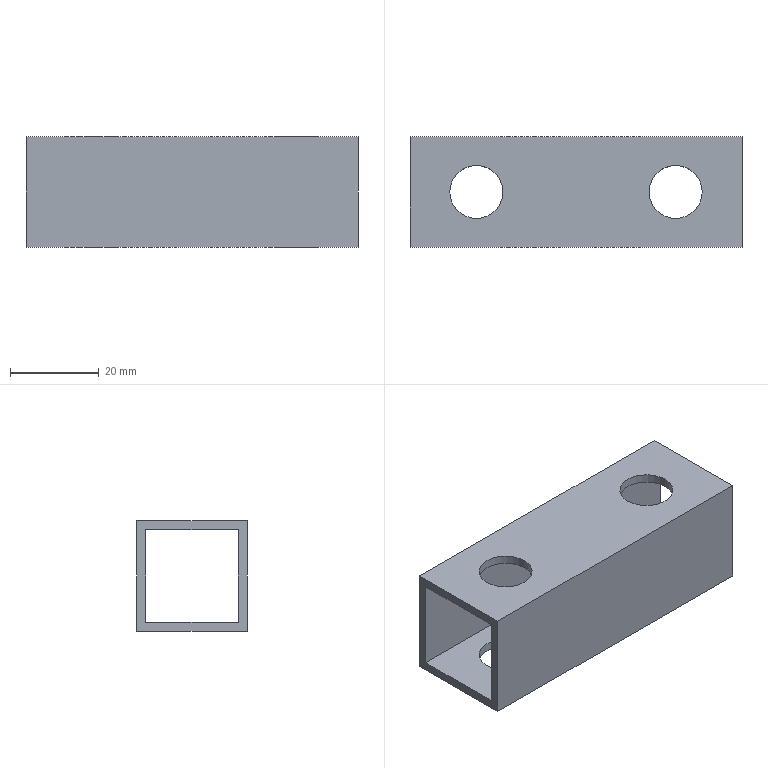Part | NX | features solid 2 | 1 solid | 14 faces | box 75 x 25 x 25 mm | volume 12895 mm3 | plane 10 | cylinder 4 | commonest cylinder face diameters 12 x4
STEP:
#1=CARTESIAN_POINT('',(-690.,-237.5,-30.));
#2=VERTEX_POINT('',#1);
#3=CARTESIAN_POINT('',(-615.,-237.5,-30.));
#4=VERTEX_POINT('',#3);
#5=CARTESIAN_POINT('',(-690.,-237.5,-30.));
#6=DIRECTION('',(1.,0.,0.));
#7=VECTOR('',#6,1000.);
#8=LINE('',#5,#7);
#9=EDGE_CURVE('',#2,#4,#8,.T.);
#10=ORIENTED_EDGE('',*,*,#9,.F.);
#11=CARTESIAN_POINT('',(-690.,-262.5,-30.));
#12=VERTEX_POINT('',#11);
#13=CARTESIAN_POINT('',(-690.,-262.5,-30.));
#14=DIRECTION('',(0.,1.,0.));
#15=VECTOR('',#14,1000.);
#16=LINE('',#13,#15);
#17=EDGE_CURVE('',#12,#2,#16,.T.);
#18=ORIENTED_EDGE('',*,*,#17,.F.);
#19=CARTESIAN_POINT('',(-615.,-262.5,-30.));
#20=VERTEX_POINT('',#19);
#21=CARTESIAN_POINT('',(-690.,-262.5,-30.));
#22=DIRECTION('',(1.,0.,0.));
#23=VECTOR('',#22,1000.);
#24=LINE('',#21,#23);
#25=EDGE_CURVE('',#12,#20,#24,.T.);
#26=ORIENTED_EDGE('',*,*,#25,.T.);
#27=CARTESIAN_POINT('',(-615.,-262.5,-30.));
#28=DIRECTION('',(0.,-1.,0.));
#29=VECTOR('',#28,1000.);
#30=LINE('',#27,#29);
#31=EDGE_CURVE('',#20,#4,#30,.F.);
#32=ORIENTED_EDGE('',*,*,#31,.T.);
#33=EDGE_LOOP('',(#10,#18,#26,#32));
#34=FACE_BOUND('',#33,.T.);
#35=CARTESIAN_POINT('',(-669.,-250.,-30.));
#36=VERTEX_POINT('',#35);
#37=CARTESIAN_POINT('',(-675.,-250.,-30.));
#38=DIRECTION('',(0.,0.,1.));
#39=DIRECTION('',(1.,0.,0.));
#40=AXIS2_PLACEMENT_3D('',#37,#38,#39);
#41=CIRCLE('',#40,6.);
#42=EDGE_CURVE('',#36,#36,#41,.T.);
#43=ORIENTED_EDGE('',*,*,#42,.F.);
#44=EDGE_LOOP('',(#43));
#45=FACE_BOUND('',#44,.T.);
#46=CARTESIAN_POINT('',(-624.,-250.,-30.));
#47=VERTEX_POINT('',#46);
#48=CARTESIAN_POINT('',(-630.,-250.,-30.));
#49=DIRECTION('',(0.,0.,1.));
#50=DIRECTION('',(1.,0.,0.));
#51=AXIS2_PLACEMENT_3D('',#48,#49,#50);
#52=CIRCLE('',#51,6.);
#53=EDGE_CURVE('',#47,#47,#52,.F.);
#54=ORIENTED_EDGE('',*,*,#53,.T.);
#55=EDGE_LOOP('',(#54));
#56=FACE_BOUND('',#55,.T.);
#57=CARTESIAN_POINT('',(-690.,-262.5,-30.));
#58=DIRECTION('',(0.,0.,1.));
#59=DIRECTION('',(1.,0.,0.));
#60=AXIS2_PLACEMENT_3D('',#57,#58,#59);
#61=PLANE('',#60);
#62=ADVANCED_FACE('',(#34,#45,#56),#61,.T.);
#63=CARTESIAN_POINT('',(-690.,-237.5,-55.));
#64=VERTEX_POINT('',#63);
#65=CARTESIAN_POINT('',(-615.,-237.5,-55.));
#66=VERTEX_POINT('',#65);
#67=CARTESIAN_POINT('',(-690.,-237.5,-55.));
#68=DIRECTION('',(1.,0.,0.));
#69=VECTOR('',#68,1000.);
#70=LINE('',#67,#69);
#71=EDGE_CURVE('',#64,#66,#70,.T.);
#72=ORIENTED_EDGE('',*,*,#71,.T.);
#73=CARTESIAN_POINT('',(-615.,-262.5,-55.));
#74=VERTEX_POINT('',#73);
#75=CARTESIAN_POINT('',(-615.,-262.5,-55.));
#76=DIRECTION('',(0.,-1.,0.));
#77=VECTOR('',#76,1000.);
#78=LINE('',#75,#77);
#79=EDGE_CURVE('',#74,#66,#78,.F.);
#80=ORIENTED_EDGE('',*,*,#79,.F.);
#81=CARTESIAN_POINT('',(-690.,-262.5,-55.));
#82=VERTEX_POINT('',#81);
#83=CARTESIAN_POINT('',(-690.,-262.5,-55.));
#84=DIRECTION('',(1.,0.,0.));
#85=VECTOR('',#84,1000.);
#86=LINE('',#83,#85);
#87=EDGE_CURVE('',#82,#74,#86,.T.);
#88=ORIENTED_EDGE('',*,*,#87,.F.);
#89=CARTESIAN_POINT('',(-690.,-262.5,-55.));
#90=DIRECTION('',(0.,1.,0.));
#91=VECTOR('',#90,1000.);
#92=LINE('',#89,#91);
#93=EDGE_CURVE('',#82,#64,#92,.T.);
#94=ORIENTED_EDGE('',*,*,#93,.T.);
#95=EDGE_LOOP('',(#72,#80,#88,#94));
#96=FACE_BOUND('',#95,.T.);
#97=CARTESIAN_POINT('',(-669.,-250.,-55.));
#98=VERTEX_POINT('',#97);
#99=CARTESIAN_POINT('',(-675.,-250.,-55.));
#100=DIRECTION('',(0.,0.,1.));
#101=DIRECTION('',(1.,0.,0.));
#102=AXIS2_PLACEMENT_3D('',#99,#100,#101);
#103=CIRCLE('',#102,6.);
#104=EDGE_CURVE('',#98,#98,#103,.T.);
#105=ORIENTED_EDGE('',*,*,#104,.T.);
#106=EDGE_LOOP('',(#105));
#107=FACE_BOUND('',#106,.T.);
#108=CARTESIAN_POINT('',(-624.,-250.,-55.));
#109=VERTEX_POINT('',#108);
#110=CARTESIAN_POINT('',(-630.,-250.,-55.));
#111=DIRECTION('',(0.,0.,1.));
#112=DIRECTION('',(1.,0.,0.));
#113=AXIS2_PLACEMENT_3D('',#110,#111,#112);
#114=CIRCLE('',#113,6.);
#115=EDGE_CURVE('',#109,#109,#114,.F.);
#116=ORIENTED_EDGE('',*,*,#115,.F.);
#117=EDGE_LOOP('',(#116));
#118=FACE_BOUND('',#117,.T.);
#119=CARTESIAN_POINT('',(-690.,-262.5,-55.));
#120=DIRECTION('',(0.,0.,1.));
#121=DIRECTION('',(1.,0.,0.));
#122=AXIS2_PLACEMENT_3D('',#119,#120,#121);
#123=PLANE('',#122);
#124=ADVANCED_FACE('',(#96,#107,#118),#123,.F.);
#125=CARTESIAN_POINT('',(-690.,-239.5,-32.));
#126=VERTEX_POINT('',#125);
#127=CARTESIAN_POINT('',(-615.,-239.5,-32.));
#128=VERTEX_POINT('',#127);
#129=CARTESIAN_POINT('',(-690.,-239.5,-32.));
#130=DIRECTION('',(-1.,0.,0.));
#131=VECTOR('',#130,1000.);
#132=LINE('',#129,#131);
#133=EDGE_CURVE('',#126,#128,#132,.F.);
#134=ORIENTED_EDGE('',*,*,#133,.T.);
#135=CARTESIAN_POINT('',(-615.,-260.5,-32.));
#136=VERTEX_POINT('',#135);
#137=CARTESIAN_POINT('',(-615.,-265.,-32.));
#138=DIRECTION('',(0.,1.,0.));
#139=VECTOR('',#138,1000.);
#140=LINE('',#137,#139);
#141=EDGE_CURVE('',#128,#136,#140,.F.);
#142=ORIENTED_EDGE('',*,*,#141,.T.);
#143=CARTESIAN_POINT('',(-690.,-260.5,-32.));
#144=VERTEX_POINT('',#143);
#145=CARTESIAN_POINT('',(-690.,-260.5,-32.));
#146=DIRECTION('',(1.,0.,0.));
#147=VECTOR('',#146,1000.);
#148=LINE('',#145,#147);
#149=EDGE_CURVE('',#144,#136,#148,.T.);
#150=ORIENTED_EDGE('',*,*,#149,.F.);
#151=CARTESIAN_POINT('',(-690.,-262.5,-32.));
#152=DIRECTION('',(0.,-1.,0.));
#153=VECTOR('',#152,1000.);
#154=LINE('',#151,#153);
#155=EDGE_CURVE('',#144,#126,#154,.F.);
#156=ORIENTED_EDGE('',*,*,#155,.T.);
#157=EDGE_LOOP('',(#134,#142,#150,#156));
#158=FACE_BOUND('',#157,.T.);
#159=CARTESIAN_POINT('',(-669.,-250.,-32.));
#160=VERTEX_POINT('',#159);
#161=CARTESIAN_POINT('',(-675.,-250.,-32.));
#162=DIRECTION('',(0.,0.,1.));
#163=DIRECTION('',(1.,0.,0.));
#164=AXIS2_PLACEMENT_3D('',#161,#162,#163);
#165=CIRCLE('',#164,6.);
#166=EDGE_CURVE('',#160,#160,#165,.T.);
#167=ORIENTED_EDGE('',*,*,#166,.T.);
#168=EDGE_LOOP('',(#167));
#169=FACE_BOUND('',#168,.T.);
#170=CARTESIAN_POINT('',(-624.,-250.,-32.));
#171=VERTEX_POINT('',#170);
#172=CARTESIAN_POINT('',(-630.,-250.,-32.));
#173=DIRECTION('',(0.,0.,1.));
#174=DIRECTION('',(1.,0.,0.));
#175=AXIS2_PLACEMENT_3D('',#172,#173,#174);
#176=CIRCLE('',#175,6.);
#177=EDGE_CURVE('',#171,#171,#176,.F.);
#178=ORIENTED_EDGE('',*,*,#177,.F.);
#179=EDGE_LOOP('',(#178));
#180=FACE_BOUND('',#179,.T.);
#181=CARTESIAN_POINT('',(-690.,-262.5,-32.));
#182=DIRECTION('',(0.,0.,1.));
#183=DIRECTION('',(1.,0.,0.));
#184=AXIS2_PLACEMENT_3D('',#181,#182,#183);
#185=PLANE('',#184);
#186=ADVANCED_FACE('',(#158,#169,#180),#185,.F.);
#187=CARTESIAN_POINT('',(-690.,-239.5,-53.));
#188=VERTEX_POINT('',#187);
#189=CARTESIAN_POINT('',(-615.,-239.5,-53.));
#190=VERTEX_POINT('',#189);
#191=CARTESIAN_POINT('',(-690.,-239.5,-53.));
#192=DIRECTION('',(-1.,0.,0.));
#193=VECTOR('',#192,1000.);
#194=LINE('',#191,#193);
#195=EDGE_CURVE('',#188,#190,#194,.F.);
#196=ORIENTED_EDGE('',*,*,#195,.F.);
#197=CARTESIAN_POINT('',(-690.,-260.5,-53.));
#198=VERTEX_POINT('',#197);
#199=CARTESIAN_POINT('',(-690.,-262.5,-53.));
#200=DIRECTION('',(0.,-1.,0.));
#201=VECTOR('',#200,1000.);
#202=LINE('',#199,#201);
#203=EDGE_CURVE('',#198,#188,#202,.F.);
#204=ORIENTED_EDGE('',*,*,#203,.F.);
#205=CARTESIAN_POINT('',(-615.,-260.5,-53.));
#206=VERTEX_POINT('',#205);
#207=CARTESIAN_POINT('',(-690.,-260.5,-53.));
#208=DIRECTION('',(1.,0.,0.));
#209=VECTOR('',#208,1000.);
#210=LINE('',#207,#209);
#211=EDGE_CURVE('',#198,#206,#210,.T.);
#212=ORIENTED_EDGE('',*,*,#211,.T.);
#213=CARTESIAN_POINT('',(-615.,-265.,-53.));
#214=DIRECTION('',(0.,1.,0.));
#215=VECTOR('',#214,1000.);
#216=LINE('',#213,#215);
#217=EDGE_CURVE('',#190,#206,#216,.F.);
#218=ORIENTED_EDGE('',*,*,#217,.F.);
#219=EDGE_LOOP('',(#196,#204,#212,#218));
#220=FACE_BOUND('',#219,.T.);
#221=CARTESIAN_POINT('',(-669.,-250.,-53.));
#222=VERTEX_POINT('',#221);
#223=CARTESIAN_POINT('',(-675.,-250.,-53.));
#224=DIRECTION('',(0.,0.,1.));
#225=DIRECTION('',(1.,0.,0.));
#226=AXIS2_PLACEMENT_3D('',#223,#224,#225);
#227=CIRCLE('',#226,6.);
#228=EDGE_CURVE('',#222,#222,#227,.T.);
#229=ORIENTED_EDGE('',*,*,#228,.F.);
#230=EDGE_LOOP('',(#229));
#231=FACE_BOUND('',#230,.T.);
#232=CARTESIAN_POINT('',(-624.,-250.,-53.));
#233=VERTEX_POINT('',#232);
#234=CARTESIAN_POINT('',(-630.,-250.,-53.));
#235=DIRECTION('',(0.,0.,1.));
#236=DIRECTION('',(1.,0.,0.));
#237=AXIS2_PLACEMENT_3D('',#234,#235,#236);
#238=CIRCLE('',#237,6.);
#239=EDGE_CURVE('',#233,#233,#238,.F.);
#240=ORIENTED_EDGE('',*,*,#239,.T.);
#241=EDGE_LOOP('',(#240));
#242=FACE_BOUND('',#241,.T.);
#243=CARTESIAN_POINT('',(-690.,-262.5,-53.));
#244=DIRECTION('',(0.,0.,1.));
#245=DIRECTION('',(1.,0.,0.));
#246=AXIS2_PLACEMENT_3D('',#243,#244,#245);
#247=PLANE('',#246);
#248=ADVANCED_FACE('',(#220,#231,#242),#247,.T.);
#249=ORIENTED_EDGE('',*,*,#93,.F.);
#250=CARTESIAN_POINT('',(-690.,-262.5,-55.));
#251=DIRECTION('',(0.,0.,1.));
#252=VECTOR('',#251,1000.);
#253=LINE('',#250,#252);
#254=EDGE_CURVE('',#82,#12,#253,.T.);
#255=ORIENTED_EDGE('',*,*,#254,.T.);
#256=ORIENTED_EDGE('',*,*,#17,.T.);
#257=CARTESIAN_POINT('',(-690.,-237.5,-55.));
#258=DIRECTION('',(0.,0.,1.));
#259=VECTOR('',#258,1000.);
#260=LINE('',#257,#259);
#261=EDGE_CURVE('',#64,#2,#260,.T.);
#262=ORIENTED_EDGE('',*,*,#261,.F.);
#263=EDGE_LOOP('',(#249,#255,#256,#262));
#264=FACE_BOUND('',#263,.T.);
#265=CARTESIAN_POINT('',(-690.,-260.5,-55.));
#266=DIRECTION('',(0.,0.,-1.));
#267=VECTOR('',#266,1000.);
#268=LINE('',#265,#267);
#269=EDGE_CURVE('',#198,#144,#268,.F.);
#270=ORIENTED_EDGE('',*,*,#269,.F.);
#271=ORIENTED_EDGE('',*,*,#203,.T.);
#272=CARTESIAN_POINT('',(-690.,-239.5,-55.));
#273=DIRECTION('',(0.,0.,1.));
#274=VECTOR('',#273,1000.);
#275=LINE('',#272,#274);
#276=EDGE_CURVE('',#188,#126,#275,.T.);
#277=ORIENTED_EDGE('',*,*,#276,.T.);
#278=ORIENTED_EDGE('',*,*,#155,.F.);
#279=EDGE_LOOP('',(#270,#271,#277,#278));
#280=FACE_BOUND('',#279,.T.);
#281=CARTESIAN_POINT('',(-690.,-262.5,-55.));
#282=DIRECTION('',(1.,0.,0.));
#283=DIRECTION('',(0.,1.,0.));
#284=AXIS2_PLACEMENT_3D('',#281,#282,#283);
#285=PLANE('',#284);
#286=ADVANCED_FACE('',(#264,#280),#285,.F.);
#287=ORIENTED_EDGE('',*,*,#254,.F.);
#288=ORIENTED_EDGE('',*,*,#87,.T.);
#289=CARTESIAN_POINT('',(-615.,-262.5,-55.));
#290=DIRECTION('',(0.,0.,-1.));
#291=VECTOR('',#290,1000.);
#292=LINE('',#289,#291);
#293=EDGE_CURVE('',#74,#20,#292,.F.);
#294=ORIENTED_EDGE('',*,*,#293,.T.);
#295=ORIENTED_EDGE('',*,*,#25,.F.);
#296=EDGE_LOOP('',(#287,#288,#294,#295));
#297=FACE_BOUND('',#296,.T.);
#298=CARTESIAN_POINT('',(-690.,-262.5,-55.));
#299=DIRECTION('',(0.,-1.,0.));
#300=DIRECTION('',(1.,0.,0.));
#301=AXIS2_PLACEMENT_3D('',#298,#299,#300);
#302=PLANE('',#301);
#303=ADVANCED_FACE('',(#297),#302,.T.);
#304=CARTESIAN_POINT('',(-615.,-260.5,-55.));
#305=DIRECTION('',(0.,0.,1.));
#306=VECTOR('',#305,1000.);
#307=LINE('',#304,#306);
#308=EDGE_CURVE('',#136,#206,#307,.F.);
#309=ORIENTED_EDGE('',*,*,#308,.F.);
#310=ORIENTED_EDGE('',*,*,#141,.F.);
#311=CARTESIAN_POINT('',(-615.,-239.5,-55.));
#312=DIRECTION('',(0.,0.,-1.));
#313=VECTOR('',#312,1000.);
#314=LINE('',#311,#313);
#315=EDGE_CURVE('',#128,#190,#314,.T.);
#316=ORIENTED_EDGE('',*,*,#315,.T.);
#317=ORIENTED_EDGE('',*,*,#217,.T.);
#318=EDGE_LOOP('',(#309,#310,#316,#317));
#319=FACE_BOUND('',#318,.T.);
#320=ORIENTED_EDGE('',*,*,#293,.F.);
#321=ORIENTED_EDGE('',*,*,#79,.T.);
#322=CARTESIAN_POINT('',(-615.,-237.5,-55.));
#323=DIRECTION('',(0.,0.,1.));
#324=VECTOR('',#323,1000.);
#325=LINE('',#322,#324);
#326=EDGE_CURVE('',#66,#4,#325,.T.);
#327=ORIENTED_EDGE('',*,*,#326,.T.);
#328=ORIENTED_EDGE('',*,*,#31,.F.);
#329=EDGE_LOOP('',(#320,#321,#327,#328));
#330=FACE_BOUND('',#329,.T.);
#331=CARTESIAN_POINT('',(-615.,-265.,-55.));
#332=DIRECTION('',(-1.,0.,0.));
#333=DIRECTION('',(0.,-1.,0.));
#334=AXIS2_PLACEMENT_3D('',#331,#332,#333);
#335=PLANE('',#334);
#336=ADVANCED_FACE('',(#319,#330),#335,.F.);
#337=ORIENTED_EDGE('',*,*,#326,.F.);
#338=ORIENTED_EDGE('',*,*,#71,.F.);
#339=ORIENTED_EDGE('',*,*,#261,.T.);
#340=ORIENTED_EDGE('',*,*,#9,.T.);
#341=EDGE_LOOP('',(#337,#338,#339,#340));
#342=FACE_BOUND('',#341,.T.);
#343=CARTESIAN_POINT('',(-690.,-237.5,-55.));
#344=DIRECTION('',(0.,-1.,0.));
#345=DIRECTION('',(1.,0.,0.));
#346=AXIS2_PLACEMENT_3D('',#343,#344,#345);
#347=PLANE('',#346);
#348=ADVANCED_FACE('',(#342),#347,.F.);
#349=ORIENTED_EDGE('',*,*,#269,.T.);
#350=ORIENTED_EDGE('',*,*,#149,.T.);
#351=ORIENTED_EDGE('',*,*,#308,.T.);
#352=ORIENTED_EDGE('',*,*,#211,.F.);
#353=EDGE_LOOP('',(#349,#350,#351,#352));
#354=FACE_BOUND('',#353,.T.);
#355=CARTESIAN_POINT('',(-690.,-260.5,-55.));
#356=DIRECTION('',(0.,-1.,0.));
#357=DIRECTION('',(1.,0.,0.));
#358=AXIS2_PLACEMENT_3D('',#355,#356,#357);
#359=PLANE('',#358);
#360=ADVANCED_FACE('',(#354),#359,.F.);
#361=ORIENTED_EDGE('',*,*,#195,.T.);
#362=ORIENTED_EDGE('',*,*,#315,.F.);
#363=ORIENTED_EDGE('',*,*,#133,.F.);
#364=ORIENTED_EDGE('',*,*,#276,.F.);
#365=EDGE_LOOP('',(#361,#362,#363,#364));
#366=FACE_BOUND('',#365,.T.);
#367=CARTESIAN_POINT('',(-690.,-239.5,-55.));
#368=DIRECTION('',(0.,-1.,0.));
#369=DIRECTION('',(1.,0.,0.));
#370=AXIS2_PLACEMENT_3D('',#367,#368,#369);
#371=PLANE('',#370);
#372=ADVANCED_FACE('',(#366),#371,.T.);
#373=ORIENTED_EDGE('',*,*,#228,.T.);
#374=EDGE_LOOP('',(#373));
#375=FACE_BOUND('',#374,.T.);
#376=ORIENTED_EDGE('',*,*,#104,.F.);
#377=EDGE_LOOP('',(#376));
#378=FACE_BOUND('',#377,.T.);
#379=CARTESIAN_POINT('',(-675.,-250.,-555.));
#380=DIRECTION('',(0.,0.,1.));
#381=DIRECTION('',(1.,0.,0.));
#382=AXIS2_PLACEMENT_3D('',#379,#380,#381);
#383=CYLINDRICAL_SURFACE('',#382,6.);
#384=ADVANCED_FACE('',(#375,#378),#383,.F.);
#385=ORIENTED_EDGE('',*,*,#42,.T.);
#386=EDGE_LOOP('',(#385));
#387=FACE_BOUND('',#386,.T.);
#388=ORIENTED_EDGE('',*,*,#166,.F.);
#389=EDGE_LOOP('',(#388));
#390=FACE_BOUND('',#389,.T.);
#391=CARTESIAN_POINT('',(-675.,-250.,-555.));
#392=DIRECTION('',(0.,0.,1.));
#393=DIRECTION('',(1.,0.,0.));
#394=AXIS2_PLACEMENT_3D('',#391,#392,#393);
#395=CYLINDRICAL_SURFACE('',#394,6.);
#396=ADVANCED_FACE('',(#387,#390),#395,.F.);
#397=ORIENTED_EDGE('',*,*,#239,.F.);
#398=EDGE_LOOP('',(#397));
#399=FACE_BOUND('',#398,.T.);
#400=ORIENTED_EDGE('',*,*,#115,.T.);
#401=EDGE_LOOP('',(#400));
#402=FACE_BOUND('',#401,.T.);
#403=CARTESIAN_POINT('',(-630.,-250.,-555.));
#404=DIRECTION('',(0.,0.,1.));
#405=DIRECTION('',(1.,0.,0.));
#406=AXIS2_PLACEMENT_3D('',#403,#404,#405);
#407=CYLINDRICAL_SURFACE('',#406,6.);
#408=ADVANCED_FACE('',(#399,#402),#407,.F.);
#409=ORIENTED_EDGE('',*,*,#53,.F.);
#410=EDGE_LOOP('',(#409));
#411=FACE_BOUND('',#410,.T.);
#412=ORIENTED_EDGE('',*,*,#177,.T.);
#413=EDGE_LOOP('',(#412));
#414=FACE_BOUND('',#413,.T.);
#415=CARTESIAN_POINT('',(-630.,-250.,-555.));
#416=DIRECTION('',(0.,0.,1.));
#417=DIRECTION('',(1.,0.,0.));
#418=AXIS2_PLACEMENT_3D('',#415,#416,#417);
#419=CYLINDRICAL_SURFACE('',#418,6.);
#420=ADVANCED_FACE('',(#411,#414),#419,.F.);
#421=CLOSED_SHELL('',(#62,#124,#186,#248,#286,#303,#336,#348,#360,#372,#384,#396,#408,#420));
#422=MANIFOLD_SOLID_BREP('',#421);
#423=(LENGTH_UNIT()NAMED_UNIT(*)SI_UNIT(.MILLI.,.METRE.));
#424=UNCERTAINTY_MEASURE_WITH_UNIT(LENGTH_MEASURE(0.00001),#423,'','');
#425=(NAMED_UNIT(*)PLANE_ANGLE_UNIT()SI_UNIT($,.RADIAN.));
#426=(NAMED_UNIT(*)SI_UNIT($,.STERADIAN.)SOLID_ANGLE_UNIT());
#427=(GEOMETRIC_REPRESENTATION_CONTEXT(3)GLOBAL_UNCERTAINTY_ASSIGNED_CONTEXT((#424))GLOBAL_UNIT_ASSIGNED_CONTEXT((#423,#425,#426))REPRESENTATION_CONTEXT('',''));
#428=ADVANCED_BREP_SHAPE_REPRESENTATION('',(#422),#427);